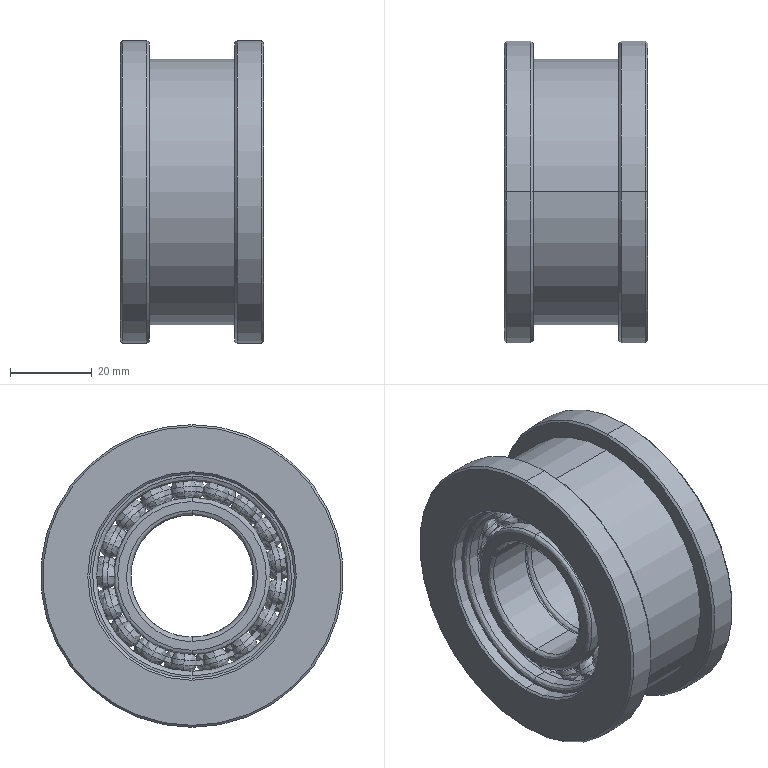Part | SolidWorks | 39 solids | 451 faces | box 35 x 74 x 74 mm | volume 78913 mm3 | spline 186 | cylinder 170 | plane 83 | cone 12 | commonest cylinder face diameters 41.25 x66 43.75 x66 38.333 x8 46.667 x8 55 x8 30 x4